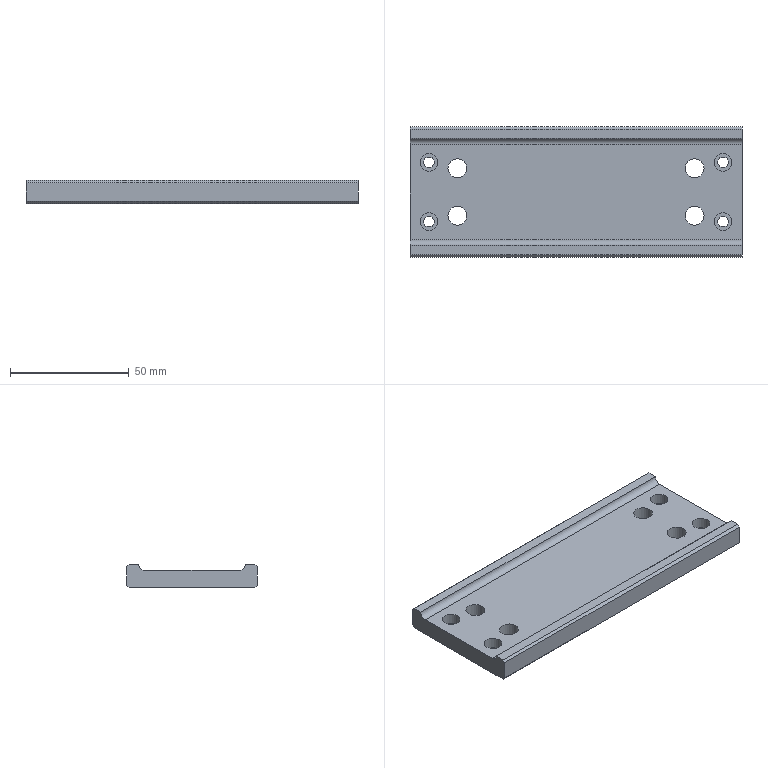Part | STEP file | Tube necking machine_id74_x_t | 1 solid | 30 faces | box 140 x 55 x 10 mm | volume 58161 mm3 | plane 16 | cylinder 14 | commonest cylinder face diameters 4.5 x4 7.5 x4 8 x4 5.2 x2